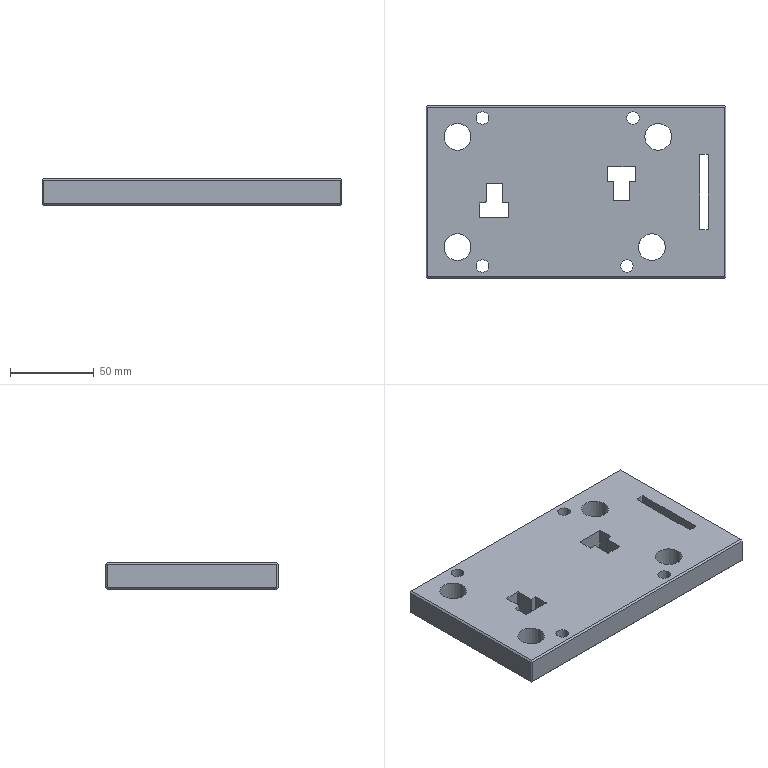Part | Creo | features DATUM PLANE 3, CURVE 2, PROTRUSION 2, CHAMFER 1, COORDINATE SYSTEM 1 | 1 solid | 98 faces | box 179.25 x 103.5 x 16 mm | volume 267287 mm3 | cylinder 52 | plane 46 | commonest cylinder face diameters 0.75 x16 4.5 x16 7.5 x8 16 x8 1.5 x4